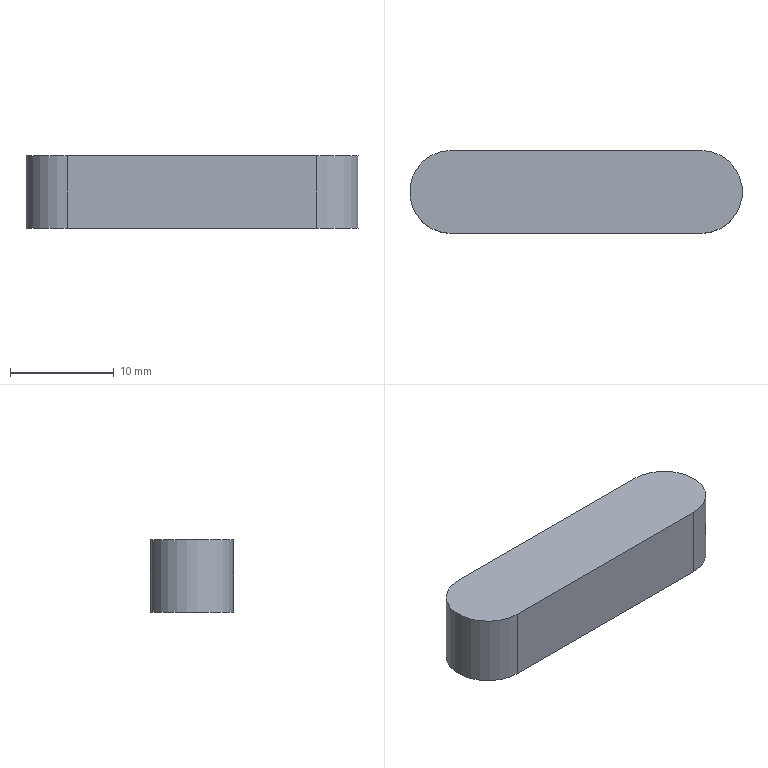Part | NX | features DATUM_CSYS 2, EXTRUDE 1, SKETCH 1 | 1 solid | 6 faces | box 32 x 8 x 7 mm | volume 1696 mm3 | plane 4 | cylinder 2 | commonest cylinder face diameters 8 x2
STEP:
#1=CARTESIAN_POINT('',(0.,4.,0.));
#2=VERTEX_POINT('',#1);
#3=CARTESIAN_POINT('',(0.,-4.,0.));
#4=VERTEX_POINT('',#3);
#5=CARTESIAN_POINT('',(0.,0.,0.));
#6=DIRECTION('',(0.,0.,1.));
#7=DIRECTION('',(1.,0.,0.));
#8=AXIS2_PLACEMENT_3D('',#5,#6,#7);
#9=CIRCLE('',#8,4.);
#10=EDGE_CURVE('',#2,#4,#9,.T.);
#11=ORIENTED_EDGE('',*,*,#10,.T.);
#12=CARTESIAN_POINT('',(0.,-4.,7.));
#13=VERTEX_POINT('',#12);
#14=CARTESIAN_POINT('',(0.,-4.,7.));
#15=DIRECTION('',(0.,0.,-1.));
#16=VECTOR('',#15,1000.);
#17=LINE('',#14,#16);
#18=EDGE_CURVE('',#13,#4,#17,.T.);
#19=ORIENTED_EDGE('',*,*,#18,.F.);
#20=CARTESIAN_POINT('',(0.,4.,7.));
#21=VERTEX_POINT('',#20);
#22=CARTESIAN_POINT('',(0.,0.,7.));
#23=DIRECTION('',(0.,0.,1.));
#24=DIRECTION('',(1.,0.,0.));
#25=AXIS2_PLACEMENT_3D('',#22,#23,#24);
#26=CIRCLE('',#25,4.);
#27=EDGE_CURVE('',#21,#13,#26,.T.);
#28=ORIENTED_EDGE('',*,*,#27,.F.);
#29=CARTESIAN_POINT('',(0.,4.,7.));
#30=DIRECTION('',(0.,0.,-1.));
#31=VECTOR('',#30,1000.);
#32=LINE('',#29,#31);
#33=EDGE_CURVE('',#21,#2,#32,.T.);
#34=ORIENTED_EDGE('',*,*,#33,.T.);
#35=EDGE_LOOP('',(#11,#19,#28,#34));
#36=FACE_BOUND('',#35,.T.);
#37=CARTESIAN_POINT('',(0.,0.,7.));
#38=DIRECTION('',(0.,0.,-1.));
#39=DIRECTION('',(-1.,0.,0.));
#40=AXIS2_PLACEMENT_3D('',#37,#38,#39);
#41=CYLINDRICAL_SURFACE('',#40,4.);
#42=ADVANCED_FACE('',(#36),#41,.T.);
#43=CARTESIAN_POINT('',(24.,-4.,0.));
#44=VERTEX_POINT('',#43);
#45=CARTESIAN_POINT('',(0.,-4.,0.));
#46=DIRECTION('',(1.,0.,0.));
#47=VECTOR('',#46,1000.);
#48=LINE('',#45,#47);
#49=EDGE_CURVE('',#4,#44,#48,.T.);
#50=ORIENTED_EDGE('',*,*,#49,.T.);
#51=CARTESIAN_POINT('',(24.,-4.,7.));
#52=VERTEX_POINT('',#51);
#53=CARTESIAN_POINT('',(24.,-4.,7.));
#54=DIRECTION('',(0.,0.,-1.));
#55=VECTOR('',#54,1000.);
#56=LINE('',#53,#55);
#57=EDGE_CURVE('',#52,#44,#56,.T.);
#58=ORIENTED_EDGE('',*,*,#57,.F.);
#59=CARTESIAN_POINT('',(0.,-4.,7.));
#60=DIRECTION('',(1.,0.,0.));
#61=VECTOR('',#60,1000.);
#62=LINE('',#59,#61);
#63=EDGE_CURVE('',#13,#52,#62,.T.);
#64=ORIENTED_EDGE('',*,*,#63,.F.);
#65=ORIENTED_EDGE('',*,*,#18,.T.);
#66=EDGE_LOOP('',(#50,#58,#64,#65));
#67=FACE_BOUND('',#66,.T.);
#68=CARTESIAN_POINT('',(0.,-4.,7.));
#69=DIRECTION('',(0.,1.,0.));
#70=DIRECTION('',(-1.,0.,0.));
#71=AXIS2_PLACEMENT_3D('',#68,#69,#70);
#72=PLANE('',#71);
#73=ADVANCED_FACE('',(#67),#72,.F.);
#74=CARTESIAN_POINT('',(24.,4.,0.));
#75=VERTEX_POINT('',#74);
#76=CARTESIAN_POINT('',(24.,0.,0.));
#77=DIRECTION('',(0.,0.,1.));
#78=DIRECTION('',(1.,0.,0.));
#79=AXIS2_PLACEMENT_3D('',#76,#77,#78);
#80=CIRCLE('',#79,4.);
#81=EDGE_CURVE('',#44,#75,#80,.T.);
#82=ORIENTED_EDGE('',*,*,#81,.T.);
#83=CARTESIAN_POINT('',(24.,4.,7.));
#84=VERTEX_POINT('',#83);
#85=CARTESIAN_POINT('',(24.,4.,7.));
#86=DIRECTION('',(0.,0.,-1.));
#87=VECTOR('',#86,1000.);
#88=LINE('',#85,#87);
#89=EDGE_CURVE('',#84,#75,#88,.T.);
#90=ORIENTED_EDGE('',*,*,#89,.F.);
#91=CARTESIAN_POINT('',(24.,0.,7.));
#92=DIRECTION('',(0.,0.,1.));
#93=DIRECTION('',(1.,0.,0.));
#94=AXIS2_PLACEMENT_3D('',#91,#92,#93);
#95=CIRCLE('',#94,4.);
#96=EDGE_CURVE('',#52,#84,#95,.T.);
#97=ORIENTED_EDGE('',*,*,#96,.F.);
#98=ORIENTED_EDGE('',*,*,#57,.T.);
#99=EDGE_LOOP('',(#82,#90,#97,#98));
#100=FACE_BOUND('',#99,.T.);
#101=CARTESIAN_POINT('',(24.,0.,7.));
#102=DIRECTION('',(0.,0.,-1.));
#103=DIRECTION('',(-1.,0.,0.));
#104=AXIS2_PLACEMENT_3D('',#101,#102,#103);
#105=CYLINDRICAL_SURFACE('',#104,4.);
#106=ADVANCED_FACE('',(#100),#105,.T.);
#107=CARTESIAN_POINT('',(24.,4.,0.));
#108=DIRECTION('',(-1.,0.,0.));
#109=VECTOR('',#108,1000.);
#110=LINE('',#107,#109);
#111=EDGE_CURVE('',#75,#2,#110,.T.);
#112=ORIENTED_EDGE('',*,*,#111,.T.);
#113=ORIENTED_EDGE('',*,*,#33,.F.);
#114=CARTESIAN_POINT('',(24.,4.,7.));
#115=DIRECTION('',(-1.,0.,0.));
#116=VECTOR('',#115,1000.);
#117=LINE('',#114,#116);
#118=EDGE_CURVE('',#84,#21,#117,.T.);
#119=ORIENTED_EDGE('',*,*,#118,.F.);
#120=ORIENTED_EDGE('',*,*,#89,.T.);
#121=EDGE_LOOP('',(#112,#113,#119,#120));
#122=FACE_BOUND('',#121,.T.);
#123=CARTESIAN_POINT('',(24.,4.,7.));
#124=DIRECTION('',(0.,-1.,0.));
#125=DIRECTION('',(1.,0.,0.));
#126=AXIS2_PLACEMENT_3D('',#123,#124,#125);
#127=PLANE('',#126);
#128=ADVANCED_FACE('',(#122),#127,.F.);
#129=ORIENTED_EDGE('',*,*,#27,.T.);
#130=ORIENTED_EDGE('',*,*,#63,.T.);
#131=ORIENTED_EDGE('',*,*,#96,.T.);
#132=ORIENTED_EDGE('',*,*,#118,.T.);
#133=EDGE_LOOP('',(#129,#130,#131,#132));
#134=FACE_BOUND('',#133,.T.);
#135=CARTESIAN_POINT('',(0.,0.,7.));
#136=DIRECTION('',(0.,0.,1.));
#137=DIRECTION('',(1.,0.,0.));
#138=AXIS2_PLACEMENT_3D('',#135,#136,#137);
#139=PLANE('',#138);
#140=ADVANCED_FACE('',(#134),#139,.T.);
#141=ORIENTED_EDGE('',*,*,#10,.F.);
#142=ORIENTED_EDGE('',*,*,#111,.F.);
#143=ORIENTED_EDGE('',*,*,#81,.F.);
#144=ORIENTED_EDGE('',*,*,#49,.F.);
#145=EDGE_LOOP('',(#141,#142,#143,#144));
#146=FACE_BOUND('',#145,.T.);
#147=CARTESIAN_POINT('',(0.,0.,0.));
#148=DIRECTION('',(0.,0.,1.));
#149=DIRECTION('',(1.,0.,0.));
#150=AXIS2_PLACEMENT_3D('',#147,#148,#149);
#151=PLANE('',#150);
#152=ADVANCED_FACE('',(#146),#151,.F.);
#153=CLOSED_SHELL('',(#42,#73,#106,#128,#140,#152));
#154=MANIFOLD_SOLID_BREP('',#153);
#155=(LENGTH_UNIT()NAMED_UNIT(*)SI_UNIT(.MILLI.,.METRE.));
#156=UNCERTAINTY_MEASURE_WITH_UNIT(LENGTH_MEASURE(0.00001),#155,'','');
#157=(NAMED_UNIT(*)PLANE_ANGLE_UNIT()SI_UNIT($,.RADIAN.));
#158=(NAMED_UNIT(*)SI_UNIT($,.STERADIAN.)SOLID_ANGLE_UNIT());
#159=(GEOMETRIC_REPRESENTATION_CONTEXT(3)GLOBAL_UNCERTAINTY_ASSIGNED_CONTEXT((#156))GLOBAL_UNIT_ASSIGNED_CONTEXT((#155,#157,#158))REPRESENTATION_CONTEXT('',''));
#160=ADVANCED_BREP_SHAPE_REPRESENTATION('',(#154),#159);